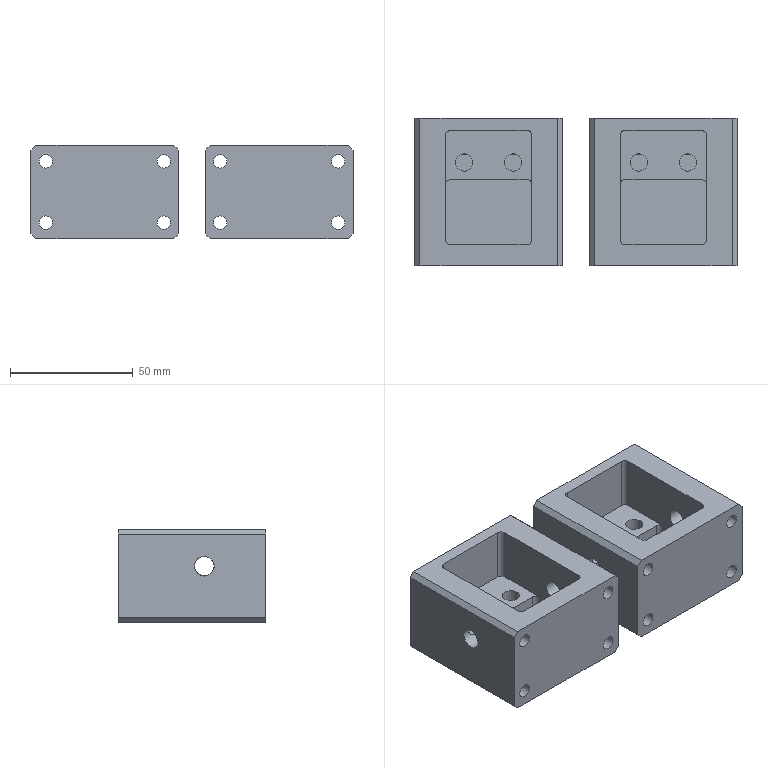CAM job | NX | 3-axis milling, drilling | part box 131 x 60 x 38 mm | stock box 136 x 65 x 40 mm
Tools:
number,name,description,diameter,corner_radius,flute_length,length,flutes
9,D10,平底铣刀-粗,10.0,0.0,35.0,75.0,2
11,D4-J,平底铣刀-精,4.0,0.0,50.0,75.0,2
10,D10-J,平底铣刀-精,10.0,0.0,35.0,75.0,2
1,D80R0.8飞刀,圆鼻刀-粗,80.0,0.8,50.0,75.0,2
1,D80R0.8飞刀-J,圆鼻刀-精,80.0,0.8,50.0,75.0,2
2,D6倒角刀,倒角刀,6.0,0.0,3.0,25.0,2
17,ZT7,钻头,7.0,0.0,35.0,50.0,2
Operations:
program,operation,operation_type,tool,method,geometry_group,spindle_rpm,surface_speed,feed_per_tooth,feed_cut,feed_plunge,cut_length_mm,path_length_mm,cut_time_min,machine_time_min
B,底壁铣飞面一刀开粗_COPY,VolumeBased25DMillingOperation,D80R0.8飞刀,分层开粗-切深K-步距G,W-B,2800.0,703.696,0.5357,3000.0,100.0,956.776,1756.734,0.3189,0.3989
B,底壁铣飞面一刀精光_COPY,VolumeBased25DMillingOperation,D80R0.8飞刀-J,侧刃精光-切深K-步距G,W-B,4000.0,1005.28,0.125,1000.0,100.0,238.998,334.998,0.239,0.2486
B,等高精光往复爬面_COPY_COPY,ZLevelMilling,D10,等高爬面-切深K-步距G,W-B,7000.0,131.947,0.3214,4500.0,100.0,3776.767,4024.331,0.8393,0.864
B,平面去毛刺6X45L_COPY,SurfaceContour,D6倒角刀,爬面_倒角-切深0-步距G,W-B,6500.0,122.519,0.1154,1500.0,100.0,241.145,652.648,0.1608,0.2019
B,底壁铣倒角_COPY_1,VolumeBased25DMillingOperation,D6倒角刀,爬面_倒角-切深0-步距G,W-B,6500.0,122.522,0.0615,800.0,100.0,286.059,727.292,0.3576,0.4017
A,顶面,FaceMilling,D80R0.8飞刀,侧刃精光-切深K-步距G,W-A,4000.0,1005.31,0.125,1000.0,100.0,225.0,261.0,0.225,0.2286
A,外形粗_2,VolumeBased25DMillingOperation,D10,METHOD,W-A,8000.0,251.327,0.3125,5000.0,80.0,27207.536,27431.236,5.441,5.464
A,台阶粗_2,CavityMilling,D10,METHOD,W-A,6000.0,188.0,0.25,3500.0,100.0,28166.829,29882.613,8.298,8.47
A,等高精光往复爬面_COPY,ZLevelMilling,D10,等高爬面-切深K-步距G,W-A,7000.0,131.947,0.3214,4500.0,100.0,3776.767,4080.598,0.8393,0.8697
A,打点-深0.8,Operation,D6倒角刀,NONE,W-A,8000.0,150.796,0.0312,500.0,90.0,7.2,192.46,0.0144,0.0329
A,盲平孔-6-8,Operation,ZT7,NONE,W-A,2200.0,48.38,0.0341,150.0,90.0,36.0,250.06,0.24,0.2614
A,清角D4,ZLevelMilling,D4-J,METHOD,W-A,6000.0,75.0,0.25,2500.0,80.0,6631.219,7152.158,2.653,2.705
A,底侧精_4,VolumeBased25DMillingOperation,D4-J,METHOD,W-A,6000.0,75.398,0.0667,800.0,100.0,741.843,1353.898,0.9273,0.9885
A,清角D4_COPY,ZLevelMilling,D4-J,METHOD,W-A,6000.0,75.0,0.25,2500.0,80.0,2402.327,2819.358,0.9618,1.004
A,底精_2,VolumeBased25DMillingOperation,D4-J,METHOD,W-A,6000.0,113.0,0.2083,1200.0,100.0,565.4,802.9,0.4712,0.4949
A,底精_1,VolumeBased25DMillingOperation,D4-J,METHOD,W-A,6000.0,113.0,0.2083,1200.0,100.0,731.161,1009.424,0.6093,0.6371
A,底侧精_3,VolumeBased25DMillingOperation,D4-J,METHOD,W-A,6000.0,113.0,0.0667,800.0,100.0,224.797,491.277,0.281,0.3076
A,底壁铣螺旋精光-中_COPY,VolumeBased25DMillingOperation,D4-J,螺旋精光-切深K-步距G,W-A,6000.0,75.398,0.0667,800.0,100.0,3098.327,3553.63,3.873,3.918
A,仅选体,SurfaceContour,D6倒角刀,METHOD,W-A,8000.0,150.796,0.1875,3000.0,100.0,744.033,1330.221,0.248,0.3066
A,铣倒角_1,PlanarMilling,D6倒角刀,METHOD,W-A,8000.0,150.796,0.05,800.0,100.0,95.661,527.197,0.1196,0.1627
A,底壁铣倒角_COPY,VolumeBased25DMillingOperation,D6倒角刀,爬面_倒角-切深0-步距G,W-A,6500.0,122.522,0.0615,800.0,100.0,286.059,547.292,0.3576,0.3837
A,底侧精_4_COPY,VolumeBased25DMillingOperation,D4-J,METHOD,W-A,6000.0,75.398,0.0667,800.0,100.0,741.843,1353.898,0.9273,0.9885
A,底侧精_3_COPY,VolumeBased25DMillingOperation,D4-J,METHOD,W-A,6000.0,113.0,0.0667,800.0,100.0,224.797,491.277,0.281,0.3076
A,外形半精_2,VolumeBased25DMillingOperation,D10-J,METHOD,W-A,8000.0,251.327,0.0625,1000.0,100.0,1121.805,1319.932,1.122,1.142